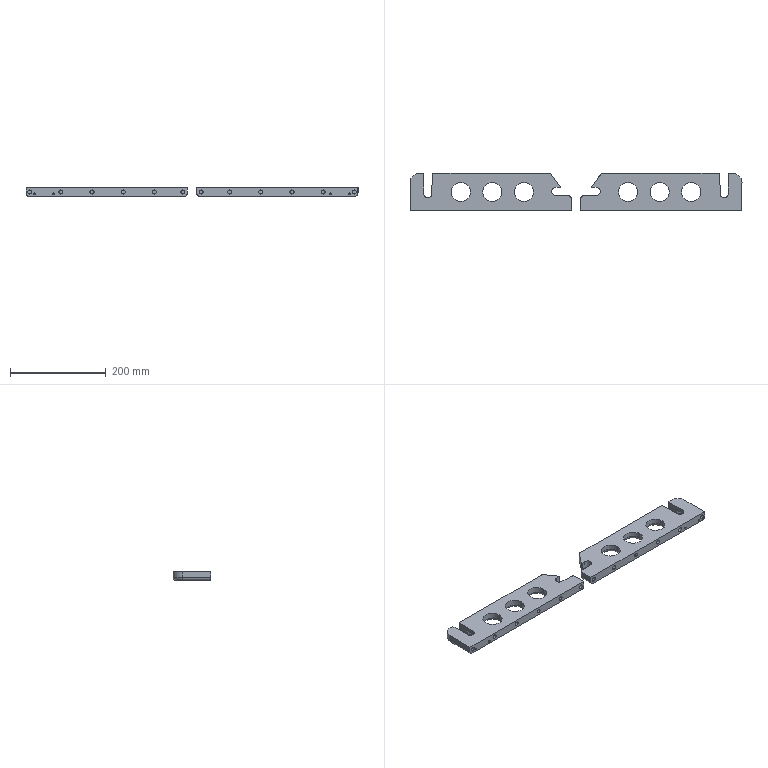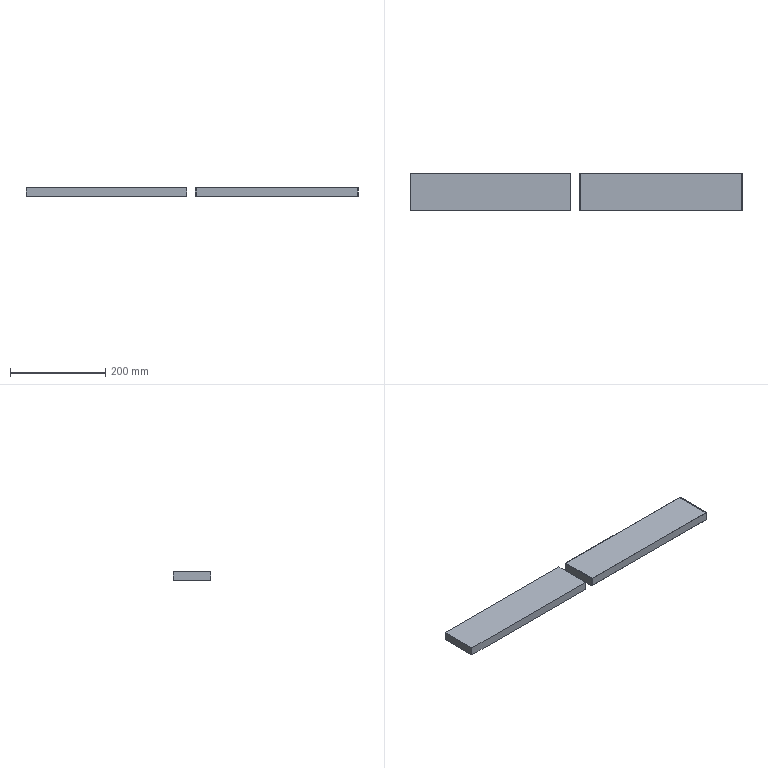CAM job | NX | 3+2 milling, drilling | part box 694.007 x 79 x 18 mm | stock box 696.007 x 79 x 18 mm
Tools:
number,name,description,diameter,corner_radius,flute_length,length,flutes
10,D10,Milling Tool-5 Parameters,10.0,0.0,50.0,75.0,2
7,D6A45,Milling Tool-5 Parameters,6.0,0.0,50.0,75.0,2
14,4.5ZT,Drilling Tool,4.5,0.0,35.0,50.0,2
11,D10JING,Milling Tool-5 Parameters,10.0,0.0,50.0,75.0,2
4,R2,Milling Tool-5 Parameters,4.0,2.0,50.0,75.0,2
5,D4R0.5,Milling Tool-5 Parameters,4.0,0.5,50.0,75.0,2
8,8.5ZT,Drilling Tool,8.5,0.0,35.0,50.0,2
9,M10,Milling Tool-5 Parameters,8.5,0.0,30.0,30.0,4
13,4.1ZT,Drilling Tool,4.0,0.0,35.0,50.0,2
12,D22内R7,User Defined Mill Tool,0.0,,8.0,51.0,2
Operations:
program,operation,operation_type,tool,method,geometry_group,spindle_rpm,surface_speed,feed_per_tooth,feed_cut,feed_plunge,cut_length_mm,path_length_mm,cut_time_min,machine_time_min
2夹,DRILLING,Operation,D6A45,METHOD,A,3000.0,56.0,0.0417,250.0,0.0,8.0,122.405,0.032,0.0434
2夹,DRILLING_COPY,Operation,4.5ZT,METHOD,A,2000.0,28.0,0.0625,250.0,0.0,24.704,155.813,0.0988,0.1119
2夹,ZLEVEL_PROFILE,ZLevelMilling,D10,METHOD,A,8000.0,251.0,0.1562,2500.0,100.0,6893.757,7540.057,2.757,2.822
2夹,HOLE_MILLING,CylinderMilling,D10,METHOD,A,8000.0,0.0,0.0,2200.0,100.0,7245.605,7878.659,3.293,3.357
2夹,HOLE_MILLING_COPY,CylinderMilling,D10JING,METHOD,A,8000.0,251.0,0.075,1200.0,100.0,510.3,1201.186,0.4252,0.4943
2夹,ZLEVEL_PROFILE_COPY_1,ZLevelMilling,D10JING,METHOD,A,8000.0,251.0,0.075,1200.0,500.0,384.444,1053.815,0.3364,0.4034
2夹,PLANAR_PROFILE,PlanarMilling,R2,METHOD,A,8000.0,100.0,0.0781,1250.0,500.0,458.328,515.36,0.3979,0.4036
2夹,PLANAR_PROFILE_2,PlanarMilling,D22内R7,METHOD,A,8000.0,0.0,0.0,1250.0,100.0,837.337,1371.661,0.6699,0.7233
2夹,PLANAR_PROFILE_2_COPY,PlanarMilling,D22内R7,METHOD,A,8000.0,0.0,0.0,1250.0,100.0,858.953,1393.722,0.6872,0.7406
2夹,PLANAR_PROFILE_2_COPY_COPY,PlanarMilling,D22内R7,METHOD,A,8000.0,0.0,0.0,1250.0,100.0,884.161,1419.171,0.7073,0.7608
2夹,ZLEVEL_PROFILE_1_COPY,ZLevelMilling,D4R0.5,METHOD,A,8000.0,100.0,0.1875,3000.0,1000.0,2318.731,2458.012,0.7785,0.7924
2夹,ZLEVEL_PROFILE_1_COPY_COPY,ZLevelMilling,D4R0.5,METHOD,A,8000.0,100.0,0.1875,3000.0,1000.0,6141.536,6252.117,2.053,2.064
1夹,ZLEVEL_PROFILE_COPY,ZLevelMilling,D10,METHOD,B,8000.0,251.0,0.1562,2500.0,100.0,712.621,1225.375,0.285,0.3363
1夹,DRILLING_COPY_1,Operation,D6A45,METHOD,B,3000.0,56.0,0.0417,250.0,0.0,32.0,467.43,0.128,0.1715
1夹,DRILLING_COPY_COPY,Operation,8.5ZT,METHOD,B,2000.0,53.0,0.0625,250.0,0.0,183.322,761.996,0.7333,0.7912
1夹,DRILLING_COPY_COPY_COPY,Operation,M10,METHOD,B,200.0,5.0,0.0019,1.5,0.0,168.0,731.352,112.0,112.056
1夹,DRILLING_COPY_COPY_1,Operation,4.1ZT,METHOD,B,2000.0,25.0,0.0375,150.0,0.0,108.403,319.919,0.7227,0.7438
22夹,DRILLING_1,Operation,D6A45,METHOD,A,3000.0,56.0,0.0417,250.0,0.0,8.0,122.405,0.032,0.0434
22夹,DRILLING_COPY_2,Operation,4.5ZT,METHOD,A,2000.0,28.0,0.0625,250.0,0.0,24.704,155.813,0.0988,0.1119
22夹,ZLEVEL_PROFILE_1,ZLevelMilling,D10,METHOD,A,8000.0,251.0,0.1562,2500.0,100.0,6893.757,7540.057,2.757,2.822
22夹,HOLE_MILLING_1,CylinderMilling,D10,METHOD,A,8000.0,0.0,0.0,2200.0,100.0,7245.605,7878.659,3.293,3.357
22夹,HOLE_MILLING_COPY_1,CylinderMilling,D10JING,METHOD,A,8000.0,251.0,0.075,1200.0,100.0,510.3,1201.711,0.4252,0.4944
22夹,ZLEVEL_PROFILE_COPY_1_1,ZLevelMilling,D10JING,METHOD,A,8000.0,251.0,0.075,1200.0,500.0,384.444,1071.116,0.3365,0.4051
22夹,PLANAR_PROFILE_1,PlanarMilling,R2,METHOD,A,8000.0,100.0,0.0781,1250.0,500.0,458.328,515.36,0.3979,0.4036
22夹,PLANAR_PROFILE_2_1,PlanarMilling,D22内R7,METHOD,A,8000.0,0.0,0.0,1250.0,100.0,837.337,1371.661,0.6699,0.7233
22夹,PLANAR_PROFILE_2_COPY_1,PlanarMilling,D22内R7,METHOD,A,8000.0,0.0,0.0,1250.0,100.0,858.953,1393.722,0.6872,0.7406
22夹,PLANAR_PROFILE_2_COPY_COPY_1,PlanarMilling,D22内R7,METHOD,A,8000.0,0.0,0.0,1250.0,100.0,884.161,1419.171,0.7073,0.7608
22夹,ZLEVEL_PROFILE_1_COPY_1,ZLevelMilling,D4R0.5,METHOD,A,8000.0,100.0,0.1875,3000.0,1000.0,2318.731,2458.012,0.7785,0.7924
22夹,ZLEVEL_PROFILE_1_COPY_COPY_1,ZLevelMilling,D4R0.5,METHOD,A,8000.0,100.0,0.1875,3000.0,1000.0,6141.861,6252.585,2.053,2.064
11夹,ZLEVEL_PROFILE_COPY_2,ZLevelMilling,D10,METHOD,B,8000.0,251.0,0.1562,2500.0,100.0,712.621,1225.375,0.285,0.3363
11夹,DRILLING_COPY_1_1,Operation,D6A45,METHOD,B,3000.0,56.0,0.0417,250.0,0.0,32.0,467.43,0.128,0.1715
11夹,DRILLING_COPY_COPY_2,Operation,8.5ZT,METHOD,B,2000.0,53.0,0.0625,250.0,0.0,183.322,761.996,0.7333,0.7912
11夹,DRILLING_COPY_COPY_COPY_1,Operation,M10,METHOD,B,200.0,5.0,0.0019,1.5,0.0,168.0,731.352,112.0,112.056
11夹,DRILLING_COPY_COPY_1_1,Operation,4.1ZT,METHOD,B,2000.0,25.0,0.0375,150.0,0.0,108.403,319.919,0.7227,0.7438